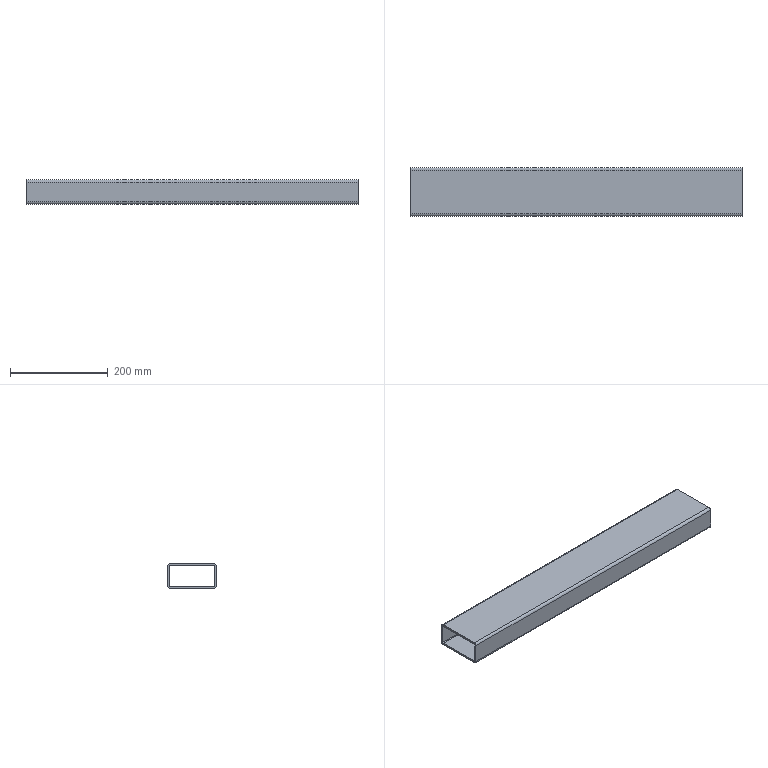Part | SolidWorks | features BaseBody 1 | 1 solid | 18 faces | box 680 x 100 x 50 mm | volume 758471 mm3 | plane 10 | cylinder 8 | commonest cylinder face diameters 2 x4 10 x4
STEP:
#1=CARTESIAN_POINT('',(-340.,45.,-25.));
#2=VERTEX_POINT('',#1);
#3=CARTESIAN_POINT('',(-340.,50.,-20.));
#4=VERTEX_POINT('',#3);
#5=CARTESIAN_POINT('',(-340.,45.,-20.));
#6=DIRECTION('',(1.,0.,0.));
#7=DIRECTION('',(0.,0.,-1.));
#8=AXIS2_PLACEMENT_3D('',#5,#6,#7);
#9=CIRCLE('',#8,5.);
#10=EDGE_CURVE('',#2,#4,#9,.T.);
#11=ORIENTED_EDGE('',*,*,#10,.T.);
#12=CARTESIAN_POINT('',(340.,50.,-20.));
#13=VERTEX_POINT('',#12);
#14=CARTESIAN_POINT('',(340.,50.,-20.));
#15=DIRECTION('',(-1.,0.,0.));
#16=VECTOR('',#15,1000.);
#17=LINE('',#14,#16);
#18=EDGE_CURVE('',#13,#4,#17,.T.);
#19=ORIENTED_EDGE('',*,*,#18,.F.);
#20=CARTESIAN_POINT('',(340.,45.,-25.));
#21=VERTEX_POINT('',#20);
#22=CARTESIAN_POINT('',(340.,45.,-20.));
#23=DIRECTION('',(1.,0.,0.));
#24=DIRECTION('',(0.,0.,-1.));
#25=AXIS2_PLACEMENT_3D('',#22,#23,#24);
#26=CIRCLE('',#25,5.);
#27=EDGE_CURVE('',#21,#13,#26,.T.);
#28=ORIENTED_EDGE('',*,*,#27,.F.);
#29=CARTESIAN_POINT('',(340.,45.,-25.));
#30=DIRECTION('',(-1.,0.,0.));
#31=VECTOR('',#30,1000.);
#32=LINE('',#29,#31);
#33=EDGE_CURVE('',#21,#2,#32,.T.);
#34=ORIENTED_EDGE('',*,*,#33,.T.);
#35=EDGE_LOOP('',(#11,#19,#28,#34));
#36=FACE_OUTER_BOUND('',#35,.T.);
#37=CARTESIAN_POINT('',(340.,45.,-20.));
#38=DIRECTION('',(-1.,0.,0.));
#39=DIRECTION('',(0.,0.,1.));
#40=AXIS2_PLACEMENT_3D('',#37,#38,#39);
#41=CYLINDRICAL_SURFACE('',#40,5.);
#42=ADVANCED_FACE('',(#36),#41,.T.);
#43=CARTESIAN_POINT('',(-340.,50.,20.));
#44=VERTEX_POINT('',#43);
#45=CARTESIAN_POINT('',(-340.,50.,-20.));
#46=DIRECTION('',(0.,0.,1.));
#47=VECTOR('',#46,1000.);
#48=LINE('',#45,#47);
#49=EDGE_CURVE('',#4,#44,#48,.T.);
#50=ORIENTED_EDGE('',*,*,#49,.T.);
#51=CARTESIAN_POINT('',(340.,50.,20.));
#52=VERTEX_POINT('',#51);
#53=CARTESIAN_POINT('',(340.,50.,20.));
#54=DIRECTION('',(-1.,0.,0.));
#55=VECTOR('',#54,1000.);
#56=LINE('',#53,#55);
#57=EDGE_CURVE('',#52,#44,#56,.T.);
#58=ORIENTED_EDGE('',*,*,#57,.F.);
#59=CARTESIAN_POINT('',(340.,50.,-20.));
#60=DIRECTION('',(0.,0.,1.));
#61=VECTOR('',#60,1000.);
#62=LINE('',#59,#61);
#63=EDGE_CURVE('',#13,#52,#62,.T.);
#64=ORIENTED_EDGE('',*,*,#63,.F.);
#65=ORIENTED_EDGE('',*,*,#18,.T.);
#66=EDGE_LOOP('',(#50,#58,#64,#65));
#67=FACE_OUTER_BOUND('',#66,.T.);
#68=CARTESIAN_POINT('',(340.,50.,-20.));
#69=DIRECTION('',(0.,-1.,0.));
#70=DIRECTION('',(0.,0.,-1.));
#71=AXIS2_PLACEMENT_3D('',#68,#69,#70);
#72=PLANE('',#71);
#73=ADVANCED_FACE('',(#67),#72,.F.);
#74=CARTESIAN_POINT('',(-340.,45.,25.));
#75=VERTEX_POINT('',#74);
#76=CARTESIAN_POINT('',(-340.,45.,20.));
#77=DIRECTION('',(1.,0.,0.));
#78=DIRECTION('',(0.,0.,-1.));
#79=AXIS2_PLACEMENT_3D('',#76,#77,#78);
#80=CIRCLE('',#79,5.);
#81=EDGE_CURVE('',#44,#75,#80,.T.);
#82=ORIENTED_EDGE('',*,*,#81,.T.);
#83=CARTESIAN_POINT('',(340.,45.,25.));
#84=VERTEX_POINT('',#83);
#85=CARTESIAN_POINT('',(340.,45.,25.));
#86=DIRECTION('',(-1.,0.,0.));
#87=VECTOR('',#86,1000.);
#88=LINE('',#85,#87);
#89=EDGE_CURVE('',#84,#75,#88,.T.);
#90=ORIENTED_EDGE('',*,*,#89,.F.);
#91=CARTESIAN_POINT('',(340.,45.,20.));
#92=DIRECTION('',(1.,0.,0.));
#93=DIRECTION('',(0.,0.,-1.));
#94=AXIS2_PLACEMENT_3D('',#91,#92,#93);
#95=CIRCLE('',#94,5.);
#96=EDGE_CURVE('',#52,#84,#95,.T.);
#97=ORIENTED_EDGE('',*,*,#96,.F.);
#98=ORIENTED_EDGE('',*,*,#57,.T.);
#99=EDGE_LOOP('',(#82,#90,#97,#98));
#100=FACE_OUTER_BOUND('',#99,.T.);
#101=CARTESIAN_POINT('',(340.,45.,20.));
#102=DIRECTION('',(-1.,0.,0.));
#103=DIRECTION('',(0.,0.,1.));
#104=AXIS2_PLACEMENT_3D('',#101,#102,#103);
#105=CYLINDRICAL_SURFACE('',#104,5.);
#106=ADVANCED_FACE('',(#100),#105,.T.);
#107=CARTESIAN_POINT('',(-340.,-45.,25.));
#108=VERTEX_POINT('',#107);
#109=CARTESIAN_POINT('',(-340.,-45.,25.));
#110=DIRECTION('',(0.,-1.,0.));
#111=VECTOR('',#110,1000.);
#112=LINE('',#109,#111);
#113=EDGE_CURVE('',#75,#108,#112,.T.);
#114=ORIENTED_EDGE('',*,*,#113,.T.);
#115=CARTESIAN_POINT('',(340.,-45.,25.));
#116=VERTEX_POINT('',#115);
#117=CARTESIAN_POINT('',(340.,-45.,25.));
#118=DIRECTION('',(-1.,0.,0.));
#119=VECTOR('',#118,1000.);
#120=LINE('',#117,#119);
#121=EDGE_CURVE('',#116,#108,#120,.T.);
#122=ORIENTED_EDGE('',*,*,#121,.F.);
#123=CARTESIAN_POINT('',(340.,-45.,25.));
#124=DIRECTION('',(0.,-1.,0.));
#125=VECTOR('',#124,1000.);
#126=LINE('',#123,#125);
#127=EDGE_CURVE('',#84,#116,#126,.T.);
#128=ORIENTED_EDGE('',*,*,#127,.F.);
#129=ORIENTED_EDGE('',*,*,#89,.T.);
#130=EDGE_LOOP('',(#114,#122,#128,#129));
#131=FACE_OUTER_BOUND('',#130,.T.);
#132=CARTESIAN_POINT('',(340.,-45.,25.));
#133=DIRECTION('',(0.,0.,-1.));
#134=DIRECTION('',(0.,1.,0.));
#135=AXIS2_PLACEMENT_3D('',#132,#133,#134);
#136=PLANE('',#135);
#137=ADVANCED_FACE('',(#131),#136,.F.);
#138=CARTESIAN_POINT('',(-340.,-50.,20.));
#139=VERTEX_POINT('',#138);
#140=CARTESIAN_POINT('',(-340.,-45.,20.));
#141=DIRECTION('',(1.,0.,0.));
#142=DIRECTION('',(0.,0.,-1.));
#143=AXIS2_PLACEMENT_3D('',#140,#141,#142);
#144=CIRCLE('',#143,5.);
#145=EDGE_CURVE('',#108,#139,#144,.T.);
#146=ORIENTED_EDGE('',*,*,#145,.T.);
#147=CARTESIAN_POINT('',(340.,-50.,20.));
#148=VERTEX_POINT('',#147);
#149=CARTESIAN_POINT('',(340.,-50.,20.));
#150=DIRECTION('',(-1.,0.,0.));
#151=VECTOR('',#150,1000.);
#152=LINE('',#149,#151);
#153=EDGE_CURVE('',#148,#139,#152,.T.);
#154=ORIENTED_EDGE('',*,*,#153,.F.);
#155=CARTESIAN_POINT('',(340.,-45.,20.));
#156=DIRECTION('',(1.,0.,0.));
#157=DIRECTION('',(0.,0.,-1.));
#158=AXIS2_PLACEMENT_3D('',#155,#156,#157);
#159=CIRCLE('',#158,5.);
#160=EDGE_CURVE('',#116,#148,#159,.T.);
#161=ORIENTED_EDGE('',*,*,#160,.F.);
#162=ORIENTED_EDGE('',*,*,#121,.T.);
#163=EDGE_LOOP('',(#146,#154,#161,#162));
#164=FACE_OUTER_BOUND('',#163,.T.);
#165=CARTESIAN_POINT('',(340.,-45.,20.));
#166=DIRECTION('',(-1.,0.,0.));
#167=DIRECTION('',(0.,0.,1.));
#168=AXIS2_PLACEMENT_3D('',#165,#166,#167);
#169=CYLINDRICAL_SURFACE('',#168,5.);
#170=ADVANCED_FACE('',(#164),#169,.T.);
#171=CARTESIAN_POINT('',(-340.,-50.,-20.));
#172=VERTEX_POINT('',#171);
#173=CARTESIAN_POINT('',(-340.,-50.,20.));
#174=DIRECTION('',(0.,0.,-1.));
#175=VECTOR('',#174,1000.);
#176=LINE('',#173,#175);
#177=EDGE_CURVE('',#139,#172,#176,.T.);
#178=ORIENTED_EDGE('',*,*,#177,.T.);
#179=CARTESIAN_POINT('',(340.,-50.,-20.));
#180=VERTEX_POINT('',#179);
#181=CARTESIAN_POINT('',(340.,-50.,-20.));
#182=DIRECTION('',(-1.,0.,0.));
#183=VECTOR('',#182,1000.);
#184=LINE('',#181,#183);
#185=EDGE_CURVE('',#180,#172,#184,.T.);
#186=ORIENTED_EDGE('',*,*,#185,.F.);
#187=CARTESIAN_POINT('',(340.,-50.,20.));
#188=DIRECTION('',(0.,0.,-1.));
#189=VECTOR('',#188,1000.);
#190=LINE('',#187,#189);
#191=EDGE_CURVE('',#148,#180,#190,.T.);
#192=ORIENTED_EDGE('',*,*,#191,.F.);
#193=ORIENTED_EDGE('',*,*,#153,.T.);
#194=EDGE_LOOP('',(#178,#186,#192,#193));
#195=FACE_OUTER_BOUND('',#194,.T.);
#196=CARTESIAN_POINT('',(340.,-50.,20.));
#197=DIRECTION('',(0.,1.,0.));
#198=DIRECTION('',(0.,0.,1.));
#199=AXIS2_PLACEMENT_3D('',#196,#197,#198);
#200=PLANE('',#199);
#201=ADVANCED_FACE('',(#195),#200,.F.);
#202=CARTESIAN_POINT('',(-340.,-45.,-25.));
#203=VERTEX_POINT('',#202);
#204=CARTESIAN_POINT('',(-340.,-45.,-20.));
#205=DIRECTION('',(1.,0.,0.));
#206=DIRECTION('',(0.,0.,-1.));
#207=AXIS2_PLACEMENT_3D('',#204,#205,#206);
#208=CIRCLE('',#207,5.);
#209=EDGE_CURVE('',#172,#203,#208,.T.);
#210=ORIENTED_EDGE('',*,*,#209,.T.);
#211=CARTESIAN_POINT('',(340.,-45.,-25.));
#212=VERTEX_POINT('',#211);
#213=CARTESIAN_POINT('',(340.,-45.,-25.));
#214=DIRECTION('',(-1.,0.,0.));
#215=VECTOR('',#214,1000.);
#216=LINE('',#213,#215);
#217=EDGE_CURVE('',#212,#203,#216,.T.);
#218=ORIENTED_EDGE('',*,*,#217,.F.);
#219=CARTESIAN_POINT('',(340.,-45.,-20.));
#220=DIRECTION('',(1.,0.,0.));
#221=DIRECTION('',(0.,0.,-1.));
#222=AXIS2_PLACEMENT_3D('',#219,#220,#221);
#223=CIRCLE('',#222,5.);
#224=EDGE_CURVE('',#180,#212,#223,.T.);
#225=ORIENTED_EDGE('',*,*,#224,.F.);
#226=ORIENTED_EDGE('',*,*,#185,.T.);
#227=EDGE_LOOP('',(#210,#218,#225,#226));
#228=FACE_OUTER_BOUND('',#227,.T.);
#229=CARTESIAN_POINT('',(340.,-45.,-20.));
#230=DIRECTION('',(-1.,0.,0.));
#231=DIRECTION('',(0.,0.,1.));
#232=AXIS2_PLACEMENT_3D('',#229,#230,#231);
#233=CYLINDRICAL_SURFACE('',#232,5.);
#234=ADVANCED_FACE('',(#228),#233,.T.);
#235=CARTESIAN_POINT('',(-340.,46.,20.));
#236=VERTEX_POINT('',#235);
#237=CARTESIAN_POINT('',(-340.,45.,21.));
#238=VERTEX_POINT('',#237);
#239=CARTESIAN_POINT('',(-340.,45.,20.));
#240=DIRECTION('',(1.,0.,0.));
#241=DIRECTION('',(0.,0.,-1.));
#242=AXIS2_PLACEMENT_3D('',#239,#240,#241);
#243=CIRCLE('',#242,1.);
#244=EDGE_CURVE('',#236,#238,#243,.T.);
#245=ORIENTED_EDGE('',*,*,#244,.F.);
#246=CARTESIAN_POINT('',(340.,46.,20.));
#247=VERTEX_POINT('',#246);
#248=CARTESIAN_POINT('',(340.,46.,20.));
#249=DIRECTION('',(-1.,0.,0.));
#250=VECTOR('',#249,1000.);
#251=LINE('',#248,#250);
#252=EDGE_CURVE('',#247,#236,#251,.T.);
#253=ORIENTED_EDGE('',*,*,#252,.F.);
#254=CARTESIAN_POINT('',(340.,45.,21.));
#255=VERTEX_POINT('',#254);
#256=CARTESIAN_POINT('',(340.,45.,20.));
#257=DIRECTION('',(1.,0.,0.));
#258=DIRECTION('',(0.,0.,-1.));
#259=AXIS2_PLACEMENT_3D('',#256,#257,#258);
#260=CIRCLE('',#259,1.);
#261=EDGE_CURVE('',#247,#255,#260,.T.);
#262=ORIENTED_EDGE('',*,*,#261,.T.);
#263=CARTESIAN_POINT('',(340.,45.,21.));
#264=DIRECTION('',(-1.,0.,0.));
#265=VECTOR('',#264,1000.);
#266=LINE('',#263,#265);
#267=EDGE_CURVE('',#255,#238,#266,.T.);
#268=ORIENTED_EDGE('',*,*,#267,.T.);
#269=EDGE_LOOP('',(#245,#253,#262,#268));
#270=FACE_OUTER_BOUND('',#269,.T.);
#271=CARTESIAN_POINT('',(340.,45.,20.));
#272=DIRECTION('',(-1.,0.,0.));
#273=DIRECTION('',(0.,0.,1.));
#274=AXIS2_PLACEMENT_3D('',#271,#272,#273);
#275=CYLINDRICAL_SURFACE('',#274,1.);
#276=ADVANCED_FACE('',(#270),#275,.F.);
#277=CARTESIAN_POINT('',(-340.,46.,-20.));
#278=VERTEX_POINT('',#277);
#279=CARTESIAN_POINT('',(-340.,46.,-20.));
#280=DIRECTION('',(0.,0.,1.));
#281=VECTOR('',#280,1000.);
#282=LINE('',#279,#281);
#283=EDGE_CURVE('',#278,#236,#282,.T.);
#284=ORIENTED_EDGE('',*,*,#283,.F.);
#285=CARTESIAN_POINT('',(340.,46.,-20.));
#286=VERTEX_POINT('',#285);
#287=CARTESIAN_POINT('',(340.,46.,-20.));
#288=DIRECTION('',(-1.,0.,0.));
#289=VECTOR('',#288,1000.);
#290=LINE('',#287,#289);
#291=EDGE_CURVE('',#286,#278,#290,.T.);
#292=ORIENTED_EDGE('',*,*,#291,.F.);
#293=CARTESIAN_POINT('',(340.,46.,-20.));
#294=DIRECTION('',(0.,0.,1.));
#295=VECTOR('',#294,1000.);
#296=LINE('',#293,#295);
#297=EDGE_CURVE('',#286,#247,#296,.T.);
#298=ORIENTED_EDGE('',*,*,#297,.T.);
#299=ORIENTED_EDGE('',*,*,#252,.T.);
#300=EDGE_LOOP('',(#284,#292,#298,#299));
#301=FACE_OUTER_BOUND('',#300,.T.);
#302=CARTESIAN_POINT('',(340.,46.,-20.));
#303=DIRECTION('',(0.,-1.,0.));
#304=DIRECTION('',(0.,0.,-1.));
#305=AXIS2_PLACEMENT_3D('',#302,#303,#304);
#306=PLANE('',#305);
#307=ADVANCED_FACE('',(#301),#306,.T.);
#308=CARTESIAN_POINT('',(-340.,45.,-21.));
#309=VERTEX_POINT('',#308);
#310=CARTESIAN_POINT('',(-340.,45.,-20.));
#311=DIRECTION('',(1.,0.,0.));
#312=DIRECTION('',(0.,0.,-1.));
#313=AXIS2_PLACEMENT_3D('',#310,#311,#312);
#314=CIRCLE('',#313,1.);
#315=EDGE_CURVE('',#309,#278,#314,.T.);
#316=ORIENTED_EDGE('',*,*,#315,.F.);
#317=CARTESIAN_POINT('',(340.,45.,-21.));
#318=VERTEX_POINT('',#317);
#319=CARTESIAN_POINT('',(340.,45.,-21.));
#320=DIRECTION('',(-1.,0.,0.));
#321=VECTOR('',#320,1000.);
#322=LINE('',#319,#321);
#323=EDGE_CURVE('',#318,#309,#322,.T.);
#324=ORIENTED_EDGE('',*,*,#323,.F.);
#325=CARTESIAN_POINT('',(340.,45.,-20.));
#326=DIRECTION('',(1.,0.,0.));
#327=DIRECTION('',(0.,0.,-1.));
#328=AXIS2_PLACEMENT_3D('',#325,#326,#327);
#329=CIRCLE('',#328,1.);
#330=EDGE_CURVE('',#318,#286,#329,.T.);
#331=ORIENTED_EDGE('',*,*,#330,.T.);
#332=ORIENTED_EDGE('',*,*,#291,.T.);
#333=EDGE_LOOP('',(#316,#324,#331,#332));
#334=FACE_OUTER_BOUND('',#333,.T.);
#335=CARTESIAN_POINT('',(340.,45.,-20.));
#336=DIRECTION('',(-1.,0.,0.));
#337=DIRECTION('',(0.,0.,1.));
#338=AXIS2_PLACEMENT_3D('',#335,#336,#337);
#339=CYLINDRICAL_SURFACE('',#338,1.);
#340=ADVANCED_FACE('',(#334),#339,.F.);
#341=CARTESIAN_POINT('',(-340.,-45.,-21.));
#342=VERTEX_POINT('',#341);
#343=CARTESIAN_POINT('',(-340.,45.,-21.));
#344=DIRECTION('',(0.,1.,0.));
#345=VECTOR('',#344,1000.);
#346=LINE('',#343,#345);
#347=EDGE_CURVE('',#342,#309,#346,.T.);
#348=ORIENTED_EDGE('',*,*,#347,.F.);
#349=CARTESIAN_POINT('',(340.,-45.,-21.));
#350=VERTEX_POINT('',#349);
#351=CARTESIAN_POINT('',(340.,-45.,-21.));
#352=DIRECTION('',(-1.,0.,0.));
#353=VECTOR('',#352,1000.);
#354=LINE('',#351,#353);
#355=EDGE_CURVE('',#350,#342,#354,.T.);
#356=ORIENTED_EDGE('',*,*,#355,.F.);
#357=CARTESIAN_POINT('',(340.,45.,-21.));
#358=DIRECTION('',(0.,1.,0.));
#359=VECTOR('',#358,1000.);
#360=LINE('',#357,#359);
#361=EDGE_CURVE('',#350,#318,#360,.T.);
#362=ORIENTED_EDGE('',*,*,#361,.T.);
#363=ORIENTED_EDGE('',*,*,#323,.T.);
#364=EDGE_LOOP('',(#348,#356,#362,#363));
#365=FACE_OUTER_BOUND('',#364,.T.);
#366=CARTESIAN_POINT('',(340.,45.,-21.));
#367=DIRECTION('',(0.,0.,1.));
#368=DIRECTION('',(1.,0.,0.));
#369=AXIS2_PLACEMENT_3D('',#366,#367,#368);
#370=PLANE('',#369);
#371=ADVANCED_FACE('',(#365),#370,.T.);
#372=CARTESIAN_POINT('',(-340.,-46.,-20.));
#373=VERTEX_POINT('',#372);
#374=CARTESIAN_POINT('',(-340.,-45.,-20.));
#375=DIRECTION('',(1.,0.,0.));
#376=DIRECTION('',(0.,0.,-1.));
#377=AXIS2_PLACEMENT_3D('',#374,#375,#376);
#378=CIRCLE('',#377,1.);
#379=EDGE_CURVE('',#373,#342,#378,.T.);
#380=ORIENTED_EDGE('',*,*,#379,.F.);
#381=CARTESIAN_POINT('',(340.,-46.,-20.));
#382=VERTEX_POINT('',#381);
#383=CARTESIAN_POINT('',(340.,-46.,-20.));
#384=DIRECTION('',(-1.,0.,0.));
#385=VECTOR('',#384,1000.);
#386=LINE('',#383,#385);
#387=EDGE_CURVE('',#382,#373,#386,.T.);
#388=ORIENTED_EDGE('',*,*,#387,.F.);
#389=CARTESIAN_POINT('',(340.,-45.,-20.));
#390=DIRECTION('',(1.,0.,0.));
#391=DIRECTION('',(0.,0.,-1.));
#392=AXIS2_PLACEMENT_3D('',#389,#390,#391);
#393=CIRCLE('',#392,1.);
#394=EDGE_CURVE('',#382,#350,#393,.T.);
#395=ORIENTED_EDGE('',*,*,#394,.T.);
#396=ORIENTED_EDGE('',*,*,#355,.T.);
#397=EDGE_LOOP('',(#380,#388,#395,#396));
#398=FACE_OUTER_BOUND('',#397,.T.);
#399=CARTESIAN_POINT('',(340.,-45.,-20.));
#400=DIRECTION('',(-1.,0.,0.));
#401=DIRECTION('',(0.,0.,1.));
#402=AXIS2_PLACEMENT_3D('',#399,#400,#401);
#403=CYLINDRICAL_SURFACE('',#402,1.);
#404=ADVANCED_FACE('',(#398),#403,.F.);
#405=CARTESIAN_POINT('',(-340.,-46.,20.));
#406=VERTEX_POINT('',#405);
#407=CARTESIAN_POINT('',(-340.,-46.,20.));
#408=DIRECTION('',(0.,0.,-1.));
#409=VECTOR('',#408,1000.);
#410=LINE('',#407,#409);
#411=EDGE_CURVE('',#406,#373,#410,.T.);
#412=ORIENTED_EDGE('',*,*,#411,.F.);
#413=CARTESIAN_POINT('',(340.,-46.,20.));
#414=VERTEX_POINT('',#413);
#415=CARTESIAN_POINT('',(340.,-46.,20.));
#416=DIRECTION('',(-1.,0.,0.));
#417=VECTOR('',#416,1000.);
#418=LINE('',#415,#417);
#419=EDGE_CURVE('',#414,#406,#418,.T.);
#420=ORIENTED_EDGE('',*,*,#419,.F.);
#421=CARTESIAN_POINT('',(340.,-46.,20.));
#422=DIRECTION('',(0.,0.,-1.));
#423=VECTOR('',#422,1000.);
#424=LINE('',#421,#423);
#425=EDGE_CURVE('',#414,#382,#424,.T.);
#426=ORIENTED_EDGE('',*,*,#425,.T.);
#427=ORIENTED_EDGE('',*,*,#387,.T.);
#428=EDGE_LOOP('',(#412,#420,#426,#427));
#429=FACE_OUTER_BOUND('',#428,.T.);
#430=CARTESIAN_POINT('',(340.,-46.,20.));
#431=DIRECTION('',(0.,1.,0.));
#432=DIRECTION('',(0.,0.,1.));
#433=AXIS2_PLACEMENT_3D('',#430,#431,#432);
#434=PLANE('',#433);
#435=ADVANCED_FACE('',(#429),#434,.T.);
#436=CARTESIAN_POINT('',(-340.,-45.,21.));
#437=VERTEX_POINT('',#436);
#438=CARTESIAN_POINT('',(-340.,-45.,20.));
#439=DIRECTION('',(1.,0.,0.));
#440=DIRECTION('',(0.,0.,-1.));
#441=AXIS2_PLACEMENT_3D('',#438,#439,#440);
#442=CIRCLE('',#441,1.);
#443=EDGE_CURVE('',#437,#406,#442,.T.);
#444=ORIENTED_EDGE('',*,*,#443,.F.);
#445=CARTESIAN_POINT('',(340.,-45.,21.));
#446=VERTEX_POINT('',#445);
#447=CARTESIAN_POINT('',(340.,-45.,21.));
#448=DIRECTION('',(-1.,0.,0.));
#449=VECTOR('',#448,1000.);
#450=LINE('',#447,#449);
#451=EDGE_CURVE('',#446,#437,#450,.T.);
#452=ORIENTED_EDGE('',*,*,#451,.F.);
#453=CARTESIAN_POINT('',(340.,-45.,20.));
#454=DIRECTION('',(1.,0.,0.));
#455=DIRECTION('',(0.,0.,-1.));
#456=AXIS2_PLACEMENT_3D('',#453,#454,#455);
#457=CIRCLE('',#456,1.);
#458=EDGE_CURVE('',#446,#414,#457,.T.);
#459=ORIENTED_EDGE('',*,*,#458,.T.);
#460=ORIENTED_EDGE('',*,*,#419,.T.);
#461=EDGE_LOOP('',(#444,#452,#459,#460));
#462=FACE_OUTER_BOUND('',#461,.T.);
#463=CARTESIAN_POINT('',(340.,-45.,20.));
#464=DIRECTION('',(-1.,0.,0.));
#465=DIRECTION('',(0.,0.,1.));
#466=AXIS2_PLACEMENT_3D('',#463,#464,#465);
#467=CYLINDRICAL_SURFACE('',#466,1.);
#468=ADVANCED_FACE('',(#462),#467,.F.);
#469=CARTESIAN_POINT('',(-340.,-45.,21.));
#470=DIRECTION('',(0.,-1.,0.));
#471=VECTOR('',#470,1000.);
#472=LINE('',#469,#471);
#473=EDGE_CURVE('',#238,#437,#472,.T.);
#474=ORIENTED_EDGE('',*,*,#473,.F.);
#475=ORIENTED_EDGE('',*,*,#267,.F.);
#476=CARTESIAN_POINT('',(340.,-45.,21.));
#477=DIRECTION('',(0.,-1.,0.));
#478=VECTOR('',#477,1000.);
#479=LINE('',#476,#478);
#480=EDGE_CURVE('',#255,#446,#479,.T.);
#481=ORIENTED_EDGE('',*,*,#480,.T.);
#482=ORIENTED_EDGE('',*,*,#451,.T.);
#483=EDGE_LOOP('',(#474,#475,#481,#482));
#484=FACE_OUTER_BOUND('',#483,.T.);
#485=CARTESIAN_POINT('',(340.,-45.,21.));
#486=DIRECTION('',(0.,0.,-1.));
#487=DIRECTION('',(0.,1.,0.));
#488=AXIS2_PLACEMENT_3D('',#485,#486,#487);
#489=PLANE('',#488);
#490=ADVANCED_FACE('',(#484),#489,.T.);
#491=CARTESIAN_POINT('',(-340.,45.,-25.));
#492=DIRECTION('',(0.,1.,0.));
#493=VECTOR('',#492,1000.);
#494=LINE('',#491,#493);
#495=EDGE_CURVE('',#203,#2,#494,.T.);
#496=ORIENTED_EDGE('',*,*,#495,.T.);
#497=ORIENTED_EDGE('',*,*,#33,.F.);
#498=CARTESIAN_POINT('',(340.,45.,-25.));
#499=DIRECTION('',(0.,1.,0.));
#500=VECTOR('',#499,1000.);
#501=LINE('',#498,#500);
#502=EDGE_CURVE('',#212,#21,#501,.T.);
#503=ORIENTED_EDGE('',*,*,#502,.F.);
#504=ORIENTED_EDGE('',*,*,#217,.T.);
#505=EDGE_LOOP('',(#496,#497,#503,#504));
#506=FACE_OUTER_BOUND('',#505,.T.);
#507=CARTESIAN_POINT('',(340.,45.,-25.));
#508=DIRECTION('',(0.,0.,1.));
#509=DIRECTION('',(1.,0.,0.));
#510=AXIS2_PLACEMENT_3D('',#507,#508,#509);
#511=PLANE('',#510);
#512=ADVANCED_FACE('',(#506),#511,.F.);
#513=ORIENTED_EDGE('',*,*,#261,.F.);
#514=ORIENTED_EDGE('',*,*,#297,.F.);
#515=ORIENTED_EDGE('',*,*,#330,.F.);
#516=ORIENTED_EDGE('',*,*,#361,.F.);
#517=ORIENTED_EDGE('',*,*,#394,.F.);
#518=ORIENTED_EDGE('',*,*,#425,.F.);
#519=ORIENTED_EDGE('',*,*,#458,.F.);
#520=ORIENTED_EDGE('',*,*,#480,.F.);
#521=EDGE_LOOP('',(#513,#514,#515,#516,#517,#518,#519,#520));
#522=FACE_BOUND('',#521,.T.);
#523=ORIENTED_EDGE('',*,*,#27,.T.);
#524=ORIENTED_EDGE('',*,*,#63,.T.);
#525=ORIENTED_EDGE('',*,*,#96,.T.);
#526=ORIENTED_EDGE('',*,*,#127,.T.);
#527=ORIENTED_EDGE('',*,*,#160,.T.);
#528=ORIENTED_EDGE('',*,*,#191,.T.);
#529=ORIENTED_EDGE('',*,*,#224,.T.);
#530=ORIENTED_EDGE('',*,*,#502,.T.);
#531=EDGE_LOOP('',(#523,#524,#525,#526,#527,#528,#529,#530));
#532=FACE_OUTER_BOUND('',#531,.T.);
#533=CARTESIAN_POINT('',(340.,45.,-20.));
#534=DIRECTION('',(1.,0.,0.));
#535=DIRECTION('',(0.,0.,-1.));
#536=AXIS2_PLACEMENT_3D('',#533,#534,#535);
#537=PLANE('',#536);
#538=ADVANCED_FACE('',(#522,#532),#537,.T.);
#539=ORIENTED_EDGE('',*,*,#244,.T.);
#540=ORIENTED_EDGE('',*,*,#473,.T.);
#541=ORIENTED_EDGE('',*,*,#443,.T.);
#542=ORIENTED_EDGE('',*,*,#411,.T.);
#543=ORIENTED_EDGE('',*,*,#379,.T.);
#544=ORIENTED_EDGE('',*,*,#347,.T.);
#545=ORIENTED_EDGE('',*,*,#315,.T.);
#546=ORIENTED_EDGE('',*,*,#283,.T.);
#547=EDGE_LOOP('',(#539,#540,#541,#542,#543,#544,#545,#546));
#548=FACE_BOUND('',#547,.T.);
#549=ORIENTED_EDGE('',*,*,#10,.F.);
#550=ORIENTED_EDGE('',*,*,#495,.F.);
#551=ORIENTED_EDGE('',*,*,#209,.F.);
#552=ORIENTED_EDGE('',*,*,#177,.F.);
#553=ORIENTED_EDGE('',*,*,#145,.F.);
#554=ORIENTED_EDGE('',*,*,#113,.F.);
#555=ORIENTED_EDGE('',*,*,#81,.F.);
#556=ORIENTED_EDGE('',*,*,#49,.F.);
#557=EDGE_LOOP('',(#549,#550,#551,#552,#553,#554,#555,#556));
#558=FACE_OUTER_BOUND('',#557,.T.);
#559=CARTESIAN_POINT('',(-340.,45.,-20.));
#560=DIRECTION('',(1.,0.,0.));
#561=DIRECTION('',(0.,0.,-1.));
#562=AXIS2_PLACEMENT_3D('',#559,#560,#561);
#563=PLANE('',#562);
#564=ADVANCED_FACE('',(#548,#558),#563,.F.);
#565=CLOSED_SHELL('',(#42,#73,#106,#137,#170,#201,#234,#276,#307,#340,#371,#404,#435,#468,#490,#512,#538,#564));
#566=MANIFOLD_SOLID_BREP('',#565);
#567=CARTESIAN_POINT('',(0.,0.,0.));
#568=DIRECTION('',(0.,0.,1.));
#569=DIRECTION('',(1.,0.,0.));
#570=AXIS2_PLACEMENT_3D('',#567,#568,#569);
#571=(LENGTH_UNIT()NAMED_UNIT(*)SI_UNIT(.MILLI.,.METRE.));
#572=UNCERTAINTY_MEASURE_WITH_UNIT(LENGTH_MEASURE(0.00001),#571,'','');
#573=(NAMED_UNIT(*)PLANE_ANGLE_UNIT()SI_UNIT($,.RADIAN.));
#574=(NAMED_UNIT(*)SI_UNIT($,.STERADIAN.)SOLID_ANGLE_UNIT());
#575=(GEOMETRIC_REPRESENTATION_CONTEXT(3)GLOBAL_UNCERTAINTY_ASSIGNED_CONTEXT((#572))GLOBAL_UNIT_ASSIGNED_CONTEXT((#571,#573,#574))REPRESENTATION_CONTEXT('',''));
#576=ADVANCED_BREP_SHAPE_REPRESENTATION('',(#566,#570),#575);